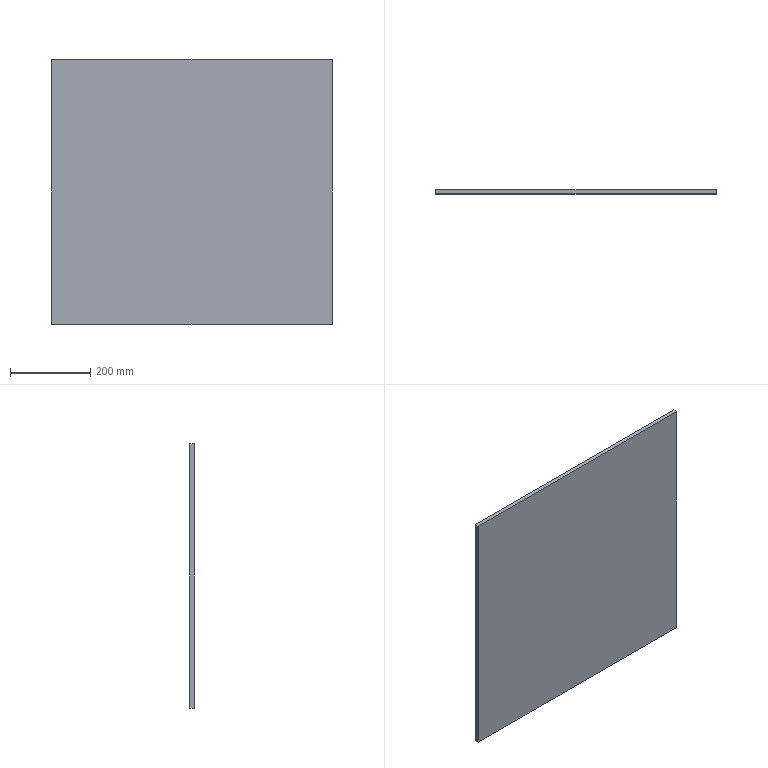Part | SolidWorks | features Extrusion 1 | 1 solid | 6 faces | box 700 x 10 x 660 mm | volume 4620000 mm3 | plane 6
STEP:
#1=CARTESIAN_POINT('',(350.,0.,-330.));
#2=VERTEX_POINT('',#1);
#3=CARTESIAN_POINT('',(-350.,0.,-330.));
#4=VERTEX_POINT('',#3);
#5=CARTESIAN_POINT('',(-350.,0.,-330.));
#6=DIRECTION('',(-1.,0.,0.));
#7=VECTOR('',#6,1000.);
#8=LINE('',#5,#7);
#9=EDGE_CURVE('',#2,#4,#8,.T.);
#10=ORIENTED_EDGE('',*,*,#9,.T.);
#11=CARTESIAN_POINT('',(-350.,10.,-330.));
#12=VERTEX_POINT('',#11);
#13=CARTESIAN_POINT('',(-350.,10.,-330.));
#14=DIRECTION('',(0.,-1.,0.));
#15=VECTOR('',#14,1000.);
#16=LINE('',#13,#15);
#17=EDGE_CURVE('',#12,#4,#16,.T.);
#18=ORIENTED_EDGE('',*,*,#17,.F.);
#19=CARTESIAN_POINT('',(350.,10.,-330.));
#20=VERTEX_POINT('',#19);
#21=CARTESIAN_POINT('',(-350.,10.,-330.));
#22=DIRECTION('',(-1.,0.,0.));
#23=VECTOR('',#22,1000.);
#24=LINE('',#21,#23);
#25=EDGE_CURVE('',#20,#12,#24,.T.);
#26=ORIENTED_EDGE('',*,*,#25,.F.);
#27=CARTESIAN_POINT('',(350.,10.,-330.));
#28=DIRECTION('',(0.,-1.,0.));
#29=VECTOR('',#28,1000.);
#30=LINE('',#27,#29);
#31=EDGE_CURVE('',#20,#2,#30,.T.);
#32=ORIENTED_EDGE('',*,*,#31,.T.);
#33=EDGE_LOOP('',(#10,#18,#26,#32));
#34=FACE_OUTER_BOUND('',#33,.T.);
#35=CARTESIAN_POINT('',(-350.,10.,-330.));
#36=DIRECTION('',(0.,0.,1.));
#37=DIRECTION('',(1.,0.,0.));
#38=AXIS2_PLACEMENT_3D('',#35,#36,#37);
#39=PLANE('',#38);
#40=ADVANCED_FACE('',(#34),#39,.F.);
#41=CARTESIAN_POINT('',(-350.,0.,330.));
#42=VERTEX_POINT('',#41);
#43=CARTESIAN_POINT('',(-350.,0.,330.));
#44=DIRECTION('',(0.,0.,1.));
#45=VECTOR('',#44,1000.);
#46=LINE('',#43,#45);
#47=EDGE_CURVE('',#4,#42,#46,.T.);
#48=ORIENTED_EDGE('',*,*,#47,.T.);
#49=CARTESIAN_POINT('',(-350.,10.,330.));
#50=VERTEX_POINT('',#49);
#51=CARTESIAN_POINT('',(-350.,10.,330.));
#52=DIRECTION('',(0.,-1.,0.));
#53=VECTOR('',#52,1000.);
#54=LINE('',#51,#53);
#55=EDGE_CURVE('',#50,#42,#54,.T.);
#56=ORIENTED_EDGE('',*,*,#55,.F.);
#57=CARTESIAN_POINT('',(-350.,10.,330.));
#58=DIRECTION('',(0.,0.,1.));
#59=VECTOR('',#58,1000.);
#60=LINE('',#57,#59);
#61=EDGE_CURVE('',#12,#50,#60,.T.);
#62=ORIENTED_EDGE('',*,*,#61,.F.);
#63=ORIENTED_EDGE('',*,*,#17,.T.);
#64=EDGE_LOOP('',(#48,#56,#62,#63));
#65=FACE_OUTER_BOUND('',#64,.T.);
#66=CARTESIAN_POINT('',(-350.,10.,330.));
#67=DIRECTION('',(1.,0.,0.));
#68=DIRECTION('',(0.,0.,-1.));
#69=AXIS2_PLACEMENT_3D('',#66,#67,#68);
#70=PLANE('',#69);
#71=ADVANCED_FACE('',(#65),#70,.F.);
#72=CARTESIAN_POINT('',(350.,0.,330.));
#73=VERTEX_POINT('',#72);
#74=CARTESIAN_POINT('',(-350.,0.,330.));
#75=DIRECTION('',(1.,0.,0.));
#76=VECTOR('',#75,1000.);
#77=LINE('',#74,#76);
#78=EDGE_CURVE('',#42,#73,#77,.T.);
#79=ORIENTED_EDGE('',*,*,#78,.T.);
#80=CARTESIAN_POINT('',(350.,10.,330.));
#81=VERTEX_POINT('',#80);
#82=CARTESIAN_POINT('',(350.,10.,330.));
#83=DIRECTION('',(0.,-1.,0.));
#84=VECTOR('',#83,1000.);
#85=LINE('',#82,#84);
#86=EDGE_CURVE('',#81,#73,#85,.T.);
#87=ORIENTED_EDGE('',*,*,#86,.F.);
#88=CARTESIAN_POINT('',(-350.,10.,330.));
#89=DIRECTION('',(1.,0.,0.));
#90=VECTOR('',#89,1000.);
#91=LINE('',#88,#90);
#92=EDGE_CURVE('',#50,#81,#91,.T.);
#93=ORIENTED_EDGE('',*,*,#92,.F.);
#94=ORIENTED_EDGE('',*,*,#55,.T.);
#95=EDGE_LOOP('',(#79,#87,#93,#94));
#96=FACE_OUTER_BOUND('',#95,.T.);
#97=CARTESIAN_POINT('',(-350.,10.,330.));
#98=DIRECTION('',(0.,0.,-1.));
#99=DIRECTION('',(-1.,0.,0.));
#100=AXIS2_PLACEMENT_3D('',#97,#98,#99);
#101=PLANE('',#100);
#102=ADVANCED_FACE('',(#96),#101,.F.);
#103=CARTESIAN_POINT('',(350.,0.,330.));
#104=DIRECTION('',(0.,0.,-1.));
#105=VECTOR('',#104,1000.);
#106=LINE('',#103,#105);
#107=EDGE_CURVE('',#73,#2,#106,.T.);
#108=ORIENTED_EDGE('',*,*,#107,.T.);
#109=ORIENTED_EDGE('',*,*,#31,.F.);
#110=CARTESIAN_POINT('',(350.,10.,330.));
#111=DIRECTION('',(0.,0.,-1.));
#112=VECTOR('',#111,1000.);
#113=LINE('',#110,#112);
#114=EDGE_CURVE('',#81,#20,#113,.T.);
#115=ORIENTED_EDGE('',*,*,#114,.F.);
#116=ORIENTED_EDGE('',*,*,#86,.T.);
#117=EDGE_LOOP('',(#108,#109,#115,#116));
#118=FACE_OUTER_BOUND('',#117,.T.);
#119=CARTESIAN_POINT('',(350.,10.,330.));
#120=DIRECTION('',(-1.,0.,0.));
#121=DIRECTION('',(0.,0.,1.));
#122=AXIS2_PLACEMENT_3D('',#119,#120,#121);
#123=PLANE('',#122);
#124=ADVANCED_FACE('',(#118),#123,.F.);
#125=ORIENTED_EDGE('',*,*,#25,.T.);
#126=ORIENTED_EDGE('',*,*,#61,.T.);
#127=ORIENTED_EDGE('',*,*,#92,.T.);
#128=ORIENTED_EDGE('',*,*,#114,.T.);
#129=EDGE_LOOP('',(#125,#126,#127,#128));
#130=FACE_OUTER_BOUND('',#129,.T.);
#131=CARTESIAN_POINT('',(0.,10.,0.));
#132=DIRECTION('',(0.,1.,0.));
#133=DIRECTION('',(0.,0.,1.));
#134=AXIS2_PLACEMENT_3D('',#131,#132,#133);
#135=PLANE('',#134);
#136=ADVANCED_FACE('',(#130),#135,.T.);
#137=ORIENTED_EDGE('',*,*,#9,.F.);
#138=ORIENTED_EDGE('',*,*,#107,.F.);
#139=ORIENTED_EDGE('',*,*,#78,.F.);
#140=ORIENTED_EDGE('',*,*,#47,.F.);
#141=EDGE_LOOP('',(#137,#138,#139,#140));
#142=FACE_OUTER_BOUND('',#141,.T.);
#143=CARTESIAN_POINT('',(0.,0.,0.));
#144=DIRECTION('',(0.,1.,0.));
#145=DIRECTION('',(0.,0.,1.));
#146=AXIS2_PLACEMENT_3D('',#143,#144,#145);
#147=PLANE('',#146);
#148=ADVANCED_FACE('',(#142),#147,.F.);
#149=CLOSED_SHELL('',(#40,#71,#102,#124,#136,#148));
#150=MANIFOLD_SOLID_BREP('',#149);
#151=CARTESIAN_POINT('',(0.,0.,0.));
#152=DIRECTION('',(0.,0.,1.));
#153=DIRECTION('',(1.,0.,0.));
#154=AXIS2_PLACEMENT_3D('',#151,#152,#153);
#155=(LENGTH_UNIT()NAMED_UNIT(*)SI_UNIT(.MILLI.,.METRE.));
#156=UNCERTAINTY_MEASURE_WITH_UNIT(LENGTH_MEASURE(0.00001),#155,'','');
#157=(NAMED_UNIT(*)PLANE_ANGLE_UNIT()SI_UNIT($,.RADIAN.));
#158=(NAMED_UNIT(*)SI_UNIT($,.STERADIAN.)SOLID_ANGLE_UNIT());
#159=(GEOMETRIC_REPRESENTATION_CONTEXT(3)GLOBAL_UNCERTAINTY_ASSIGNED_CONTEXT((#156))GLOBAL_UNIT_ASSIGNED_CONTEXT((#155,#157,#158))REPRESENTATION_CONTEXT('',''));
#160=ADVANCED_BREP_SHAPE_REPRESENTATION('',(#150,#154),#159);